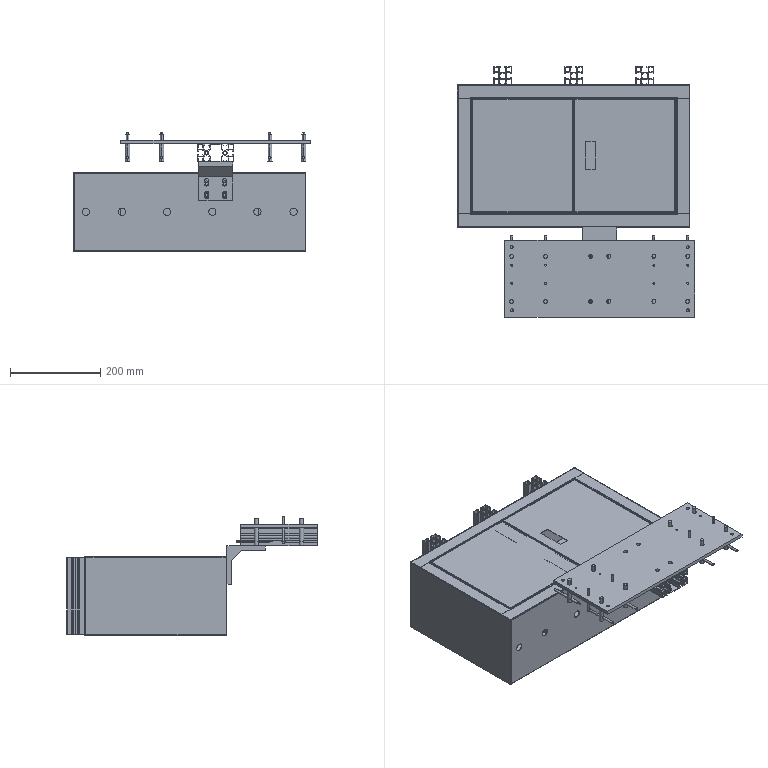Part | 38 solids | 1267 faces | box 525 x 555 x 263 mm | volume 2227239 mm3 | plane 804 | cylinder 439 | cone 16 | spline 8 | commonest cylinder face diameters 5 x40 0.2 x34 3.2 x34 10 x30 6.8 x26 3.3 x24